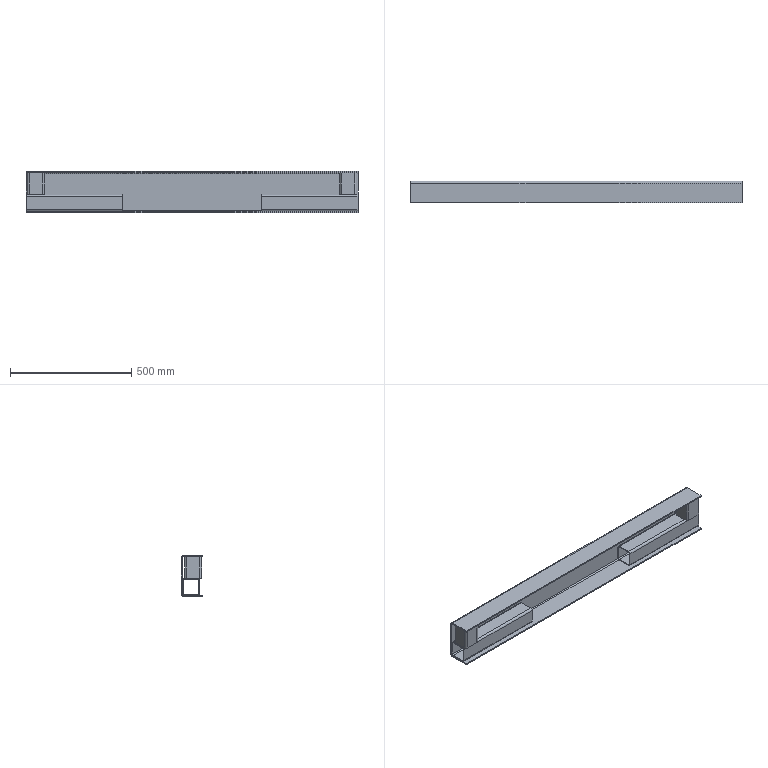Part | SolidWorks | features Cut 2, WeldMemberFeat 2, FlatPattern 1, MirrorSolid 1, SM3dBend 1, SMBaseFlange 1, SheetMetal 1, WeldmentFeature 1 | 5 solids | 110 faces | box 1370 x 90 x 169.999 mm | volume 3268075 mm3 | plane 58 | cylinder 52 | commonest cylinder face diameters 20 x18 8 x16 16 x16 10 x2